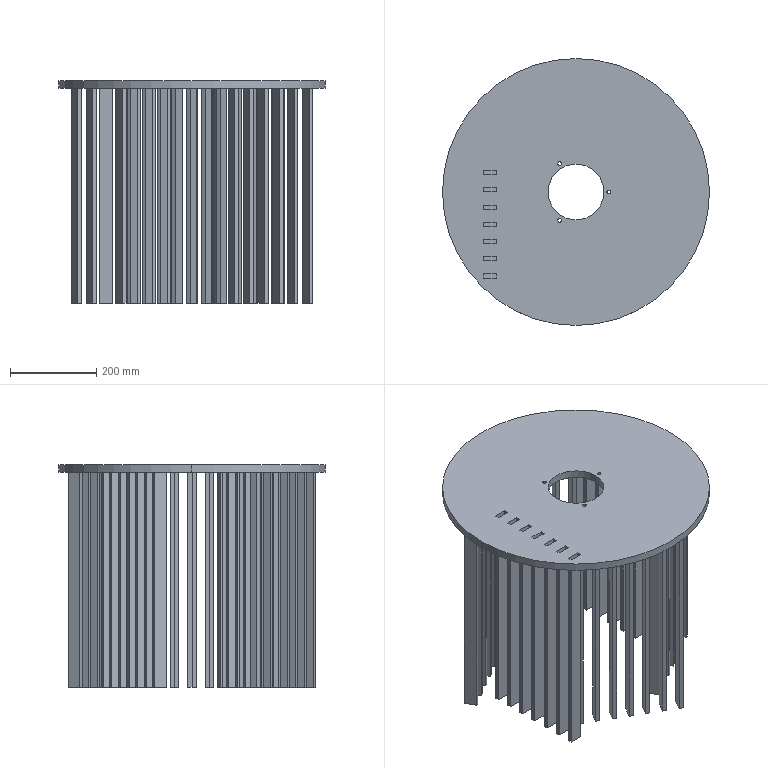Part | Creo | features PROTRUSION 7, DATUM PLANE 3, CURVE 2, COORDINATE SYSTEM 1, PATTERN 1 | 1 solid | 257 faces | box 620 x 620 x 518 mm | volume 11304252 mm3 | plane 247 | cylinder 10 | commonest cylinder face diameters 8.5 x6 130 x2 620 x2